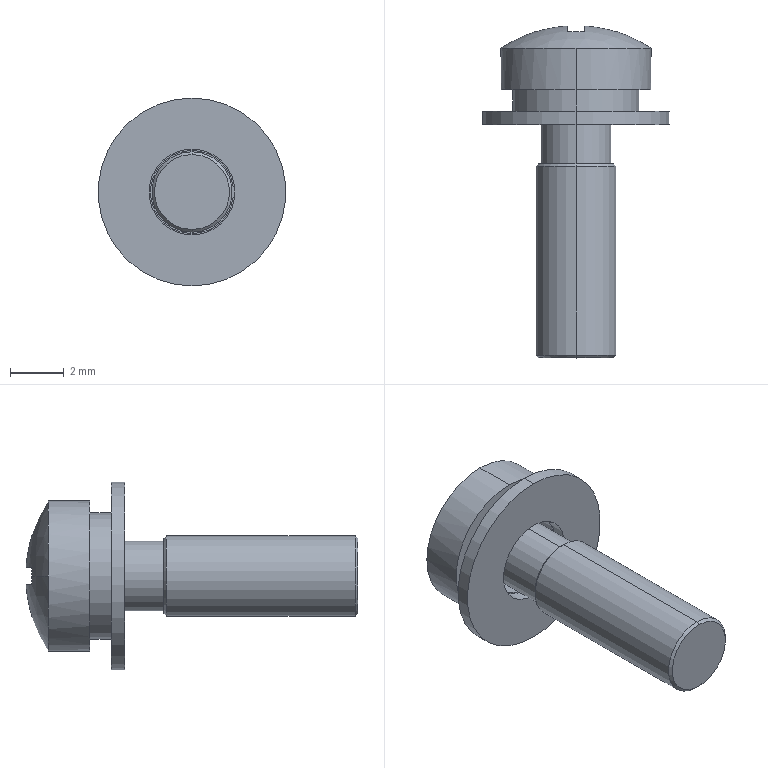Part | STEP file | 3 solids | 46 faces | box 7 x 12.378 x 7 mm | volume 131.512 mm3 | plane 22 | cylinder 16 | cone 4 | torus 2 | sphere 2 | commonest cylinder face diameters 3.1 x3 4.7 x3 2.6 x2 3 x2 3.2 x2 5.6 x2
STEP:
#1=CARTESIAN_POINT('',(0.,-12.4,-1.4));
#2=VERTEX_POINT('',#1);
#3=CARTESIAN_POINT('',(0.,-12.4,1.4));
#4=VERTEX_POINT('',#3);
#5=CARTESIAN_POINT('',(0.,-12.4,0.));
#6=DIRECTION('',(0.,-1.,0.));
#7=DIRECTION('',(0.,0.,1.));
#8=AXIS2_PLACEMENT_3D('',#5,#6,#7);
#9=CIRCLE('',#8,1.4);
#10=EDGE_CURVE('',#2,#4,#9,.T.);
#11=ORIENTED_EDGE('',*,*,#10,.F.);
#12=CARTESIAN_POINT('',(0.,-12.3,-1.5));
#13=VERTEX_POINT('',#12);
#14=CARTESIAN_POINT('',(0.,-12.4,-1.4));
#15=DIRECTION('',(0.,0.7071,-0.7071));
#16=VECTOR('',#15,1000.);
#17=LINE('',#14,#16);
#18=EDGE_CURVE('',#2,#13,#17,.T.);
#19=ORIENTED_EDGE('',*,*,#18,.T.);
#20=CARTESIAN_POINT('',(0.,-12.3,1.5));
#21=VERTEX_POINT('',#20);
#22=CARTESIAN_POINT('',(0.,-12.3,0.));
#23=DIRECTION('',(0.,1.,0.));
#24=DIRECTION('',(0.,0.,1.));
#25=AXIS2_PLACEMENT_3D('',#22,#23,#24);
#26=CIRCLE('',#25,1.5);
#27=EDGE_CURVE('',#21,#13,#26,.T.);
#28=ORIENTED_EDGE('',*,*,#27,.F.);
#29=CARTESIAN_POINT('',(0.,-12.4,1.4));
#30=DIRECTION('',(0.,0.7071,0.7071));
#31=VECTOR('',#30,1000.);
#32=LINE('',#29,#31);
#33=EDGE_CURVE('',#4,#21,#32,.T.);
#34=ORIENTED_EDGE('',*,*,#33,.F.);
#35=EDGE_LOOP('',(#11,#19,#28,#34));
#36=FACE_OUTER_BOUND('',#35,.T.);
#37=CARTESIAN_POINT('',(0.,-12.4,0.));
#38=DIRECTION('',(0.,1.,0.));
#39=DIRECTION('',(0.,0.,1.));
#40=AXIS2_PLACEMENT_3D('',#37,#38,#39);
#41=CONICAL_SURFACE('',#40,1.4,0.7854);
#42=ADVANCED_FACE('',(#36),#41,.T.);
#43=CARTESIAN_POINT('',(0.,-5.16,1.4));
#44=VERTEX_POINT('',#43);
#45=CARTESIAN_POINT('',(0.,-5.16,-1.4));
#46=VERTEX_POINT('',#45);
#47=CARTESIAN_POINT('',(0.,-5.16,0.));
#48=DIRECTION('',(0.,1.,0.));
#49=DIRECTION('',(0.,0.,1.));
#50=AXIS2_PLACEMENT_3D('',#47,#48,#49);
#51=CIRCLE('',#50,1.4);
#52=EDGE_CURVE('',#44,#46,#51,.T.);
#53=ORIENTED_EDGE('',*,*,#52,.F.);
#54=CARTESIAN_POINT('',(0.,-5.26,1.5));
#55=VERTEX_POINT('',#54);
#56=CARTESIAN_POINT('',(0.,-5.26,1.5));
#57=DIRECTION('',(0.,-0.7071,0.7071));
#58=VECTOR('',#57,1000.);
#59=LINE('',#56,#58);
#60=EDGE_CURVE('',#44,#55,#59,.T.);
#61=ORIENTED_EDGE('',*,*,#60,.T.);
#62=CARTESIAN_POINT('',(0.,-5.26,-1.5));
#63=VERTEX_POINT('',#62);
#64=CARTESIAN_POINT('',(0.,-5.26,0.));
#65=DIRECTION('',(0.,-1.,0.));
#66=DIRECTION('',(0.,0.,1.));
#67=AXIS2_PLACEMENT_3D('',#64,#65,#66);
#68=CIRCLE('',#67,1.5);
#69=EDGE_CURVE('',#63,#55,#68,.T.);
#70=ORIENTED_EDGE('',*,*,#69,.F.);
#71=CARTESIAN_POINT('',(0.,-5.26,-1.5));
#72=DIRECTION('',(0.,-0.7071,-0.7071));
#73=VECTOR('',#72,1000.);
#74=LINE('',#71,#73);
#75=EDGE_CURVE('',#46,#63,#74,.T.);
#76=ORIENTED_EDGE('',*,*,#75,.F.);
#77=EDGE_LOOP('',(#53,#61,#70,#76));
#78=FACE_OUTER_BOUND('',#77,.T.);
#79=CARTESIAN_POINT('',(0.,-5.26,0.));
#80=DIRECTION('',(0.,-1.,0.));
#81=DIRECTION('',(0.,0.,-1.));
#82=AXIS2_PLACEMENT_3D('',#79,#80,#81);
#83=CONICAL_SURFACE('',#82,1.5,0.7854);
#84=ADVANCED_FACE('',(#78),#83,.T.);
#85=CARTESIAN_POINT('',(0.,-2.5,1.3));
#86=VERTEX_POINT('',#85);
#87=CARTESIAN_POINT('',(0.,-2.5,-1.3));
#88=VERTEX_POINT('',#87);
#89=CARTESIAN_POINT('',(0.,-2.5,0.));
#90=DIRECTION('',(0.,-1.,0.));
#91=DIRECTION('',(0.,0.,-1.));
#92=AXIS2_PLACEMENT_3D('',#89,#90,#91);
#93=CIRCLE('',#92,1.3);
#94=EDGE_CURVE('',#86,#88,#93,.T.);
#95=ORIENTED_EDGE('',*,*,#94,.F.);
#96=CARTESIAN_POINT('',(0.,-2.4,1.4));
#97=VERTEX_POINT('',#96);
#98=CARTESIAN_POINT('',(0.,-2.5,1.4));
#99=DIRECTION('',(1.,0.,0.));
#100=DIRECTION('',(0.,0.,-1.));
#101=AXIS2_PLACEMENT_3D('',#98,#99,#100);
#102=CIRCLE('',#101,0.1);
#103=EDGE_CURVE('',#86,#97,#102,.T.);
#104=ORIENTED_EDGE('',*,*,#103,.T.);
#105=CARTESIAN_POINT('',(0.,-2.4,-1.4));
#106=VERTEX_POINT('',#105);
#107=CARTESIAN_POINT('',(0.,-2.4,0.));
#108=DIRECTION('',(0.,1.,0.));
#109=DIRECTION('',(0.,0.,-1.));
#110=AXIS2_PLACEMENT_3D('',#107,#108,#109);
#111=CIRCLE('',#110,1.4);
#112=EDGE_CURVE('',#106,#97,#111,.T.);
#113=ORIENTED_EDGE('',*,*,#112,.F.);
#114=CARTESIAN_POINT('',(0.,-2.5,-1.4));
#115=DIRECTION('',(-1.,0.,0.));
#116=DIRECTION('',(0.,0.,1.));
#117=AXIS2_PLACEMENT_3D('',#114,#115,#116);
#118=CIRCLE('',#117,0.1);
#119=EDGE_CURVE('',#88,#106,#118,.T.);
#120=ORIENTED_EDGE('',*,*,#119,.F.);
#121=EDGE_LOOP('',(#95,#104,#113,#120));
#122=FACE_OUTER_BOUND('',#121,.T.);
#123=CARTESIAN_POINT('',(0.,-2.5,0.));
#124=DIRECTION('',(0.,-1.,0.));
#125=DIRECTION('',(0.,0.,-1.));
#126=AXIS2_PLACEMENT_3D('',#123,#124,#125);
#127=TOROIDAL_SURFACE('',#126,1.4,0.1);
#128=ADVANCED_FACE('',(#122),#127,.F.);
#129=CARTESIAN_POINT('',(-1.5,-0.2303,0.));
#130=VERTEX_POINT('',#129);
#131=CARTESIAN_POINT('',(-1.5,-0.2421,0.335));
#132=VERTEX_POINT('',#131);
#133=CARTESIAN_POINT('',(-1.5,-5.,0.));
#134=DIRECTION('',(1.,0.,0.));
#135=DIRECTION('',(0.,0.,1.));
#136=AXIS2_PLACEMENT_3D('',#133,#134,#135);
#137=CIRCLE('',#136,4.77);
#138=EDGE_CURVE('',#130,#132,#137,.T.);
#139=ORIENTED_EDGE('',*,*,#138,.F.);
#140=CARTESIAN_POINT('',(-2.8,-0.8575,0.));
#141=VERTEX_POINT('',#140);
#142=CARTESIAN_POINT('',(0.,-5.,0.));
#143=DIRECTION('',(0.,0.,1.));
#144=DIRECTION('',(1.,0.,0.));
#145=AXIS2_PLACEMENT_3D('',#142,#143,#144);
#146=CIRCLE('',#145,5.);
#147=EDGE_CURVE('',#130,#141,#146,.T.);
#148=ORIENTED_EDGE('',*,*,#147,.T.);
#149=CARTESIAN_POINT('',(0.,-0.8575,2.8));
#150=VERTEX_POINT('',#149);
#151=CARTESIAN_POINT('',(0.,-0.8575,0.));
#152=DIRECTION('',(0.,-1.,0.));
#153=DIRECTION('',(0.,0.,-1.));
#154=AXIS2_PLACEMENT_3D('',#151,#152,#153);
#155=CIRCLE('',#154,2.8);
#156=EDGE_CURVE('',#150,#141,#155,.T.);
#157=ORIENTED_EDGE('',*,*,#156,.F.);
#158=CARTESIAN_POINT('',(2.8,-0.8575,0.));
#159=VERTEX_POINT('',#158);
#160=CARTESIAN_POINT('',(0.,-0.8575,0.));
#161=DIRECTION('',(0.,-1.,0.));
#162=DIRECTION('',(0.,0.,-1.));
#163=AXIS2_PLACEMENT_3D('',#160,#161,#162);
#164=CIRCLE('',#163,2.8);
#165=EDGE_CURVE('',#159,#150,#164,.T.);
#166=ORIENTED_EDGE('',*,*,#165,.F.);
#167=CARTESIAN_POINT('',(1.5,-0.2303,0.));
#168=VERTEX_POINT('',#167);
#169=CARTESIAN_POINT('',(0.,-5.,0.));
#170=DIRECTION('',(0.,0.,-1.));
#171=DIRECTION('',(-1.,0.,0.));
#172=AXIS2_PLACEMENT_3D('',#169,#170,#171);
#173=CIRCLE('',#172,5.);
#174=EDGE_CURVE('',#168,#159,#173,.T.);
#175=ORIENTED_EDGE('',*,*,#174,.F.);
#176=CARTESIAN_POINT('',(1.5,-0.2421,0.335));
#177=VERTEX_POINT('',#176);
#178=CARTESIAN_POINT('',(1.5,-5.,0.));
#179=DIRECTION('',(-1.,0.,0.));
#180=DIRECTION('',(0.,0.,-1.));
#181=AXIS2_PLACEMENT_3D('',#178,#179,#180);
#182=CIRCLE('',#181,4.77);
#183=EDGE_CURVE('',#177,#168,#182,.T.);
#184=ORIENTED_EDGE('',*,*,#183,.F.);
#185=CARTESIAN_POINT('',(0.335,-0.0225,0.335));
#186=VERTEX_POINT('',#185);
#187=CARTESIAN_POINT('',(0.,-5.,0.335));
#188=DIRECTION('',(0.,0.,-1.));
#189=DIRECTION('',(1.,0.,0.));
#190=AXIS2_PLACEMENT_3D('',#187,#188,#189);
#191=CIRCLE('',#190,4.989);
#192=EDGE_CURVE('',#186,#177,#191,.T.);
#193=ORIENTED_EDGE('',*,*,#192,.F.);
#194=CARTESIAN_POINT('',(0.335,-0.2421,1.5));
#195=VERTEX_POINT('',#194);
#196=CARTESIAN_POINT('',(0.335,-5.,0.));
#197=DIRECTION('',(-1.,0.,0.));
#198=DIRECTION('',(0.,0.,-1.));
#199=AXIS2_PLACEMENT_3D('',#196,#197,#198);
#200=CIRCLE('',#199,4.989);
#201=EDGE_CURVE('',#195,#186,#200,.T.);
#202=ORIENTED_EDGE('',*,*,#201,.F.);
#203=CARTESIAN_POINT('',(-0.335,-0.2421,1.5));
#204=VERTEX_POINT('',#203);
#205=CARTESIAN_POINT('',(0.,-5.,1.5));
#206=DIRECTION('',(0.,0.,-1.));
#207=DIRECTION('',(1.,0.,0.));
#208=AXIS2_PLACEMENT_3D('',#205,#206,#207);
#209=CIRCLE('',#208,4.77);
#210=EDGE_CURVE('',#204,#195,#209,.T.);
#211=ORIENTED_EDGE('',*,*,#210,.F.);
#212=CARTESIAN_POINT('',(-0.335,-0.0225,0.335));
#213=VERTEX_POINT('',#212);
#214=CARTESIAN_POINT('',(-0.335,-5.,0.));
#215=DIRECTION('',(1.,0.,0.));
#216=DIRECTION('',(0.,0.,1.));
#217=AXIS2_PLACEMENT_3D('',#214,#215,#216);
#218=CIRCLE('',#217,4.989);
#219=EDGE_CURVE('',#213,#204,#218,.T.);
#220=ORIENTED_EDGE('',*,*,#219,.F.);
#221=CARTESIAN_POINT('',(0.,-5.,0.335));
#222=DIRECTION('',(0.,0.,-1.));
#223=DIRECTION('',(1.,0.,0.));
#224=AXIS2_PLACEMENT_3D('',#221,#222,#223);
#225=CIRCLE('',#224,4.989);
#226=EDGE_CURVE('',#132,#213,#225,.T.);
#227=ORIENTED_EDGE('',*,*,#226,.F.);
#228=EDGE_LOOP('',(#139,#148,#157,#166,#175,#184,#193,#202,#211,#220,#227));
#229=FACE_OUTER_BOUND('',#228,.T.);
#230=CARTESIAN_POINT('',(0.,-5.,0.));
#231=DIRECTION('',(0.,0.,1.));
#232=DIRECTION('',(1.,0.,0.));
#233=AXIS2_PLACEMENT_3D('',#230,#231,#232);
#234=SPHERICAL_SURFACE('',#233,5.);
#235=ADVANCED_FACE('',(#229),#234,.T.);
#236=CARTESIAN_POINT('',(0.,-0.8575,-2.8));
#237=VERTEX_POINT('',#236);
#238=CARTESIAN_POINT('',(0.,-0.8575,0.));
#239=DIRECTION('',(0.,-1.,0.));
#240=DIRECTION('',(0.,0.,-1.));
#241=AXIS2_PLACEMENT_3D('',#238,#239,#240);
#242=CIRCLE('',#241,2.8);
#243=EDGE_CURVE('',#237,#159,#242,.T.);
#244=ORIENTED_EDGE('',*,*,#243,.T.);
#245=ORIENTED_EDGE('',*,*,#165,.T.);
#246=CARTESIAN_POINT('',(0.,-2.4,2.8));
#247=VERTEX_POINT('',#246);
#248=CARTESIAN_POINT('',(0.,-12.4,2.8));
#249=DIRECTION('',(0.,-1.,0.));
#250=VECTOR('',#249,1000.);
#251=LINE('',#248,#250);
#252=EDGE_CURVE('',#150,#247,#251,.T.);
#253=ORIENTED_EDGE('',*,*,#252,.T.);
#254=CARTESIAN_POINT('',(0.,-2.4,-2.8));
#255=VERTEX_POINT('',#254);
#256=CARTESIAN_POINT('',(0.,-2.4,0.));
#257=DIRECTION('',(0.,-1.,0.));
#258=DIRECTION('',(0.,0.,-1.));
#259=AXIS2_PLACEMENT_3D('',#256,#257,#258);
#260=CIRCLE('',#259,2.8);
#261=EDGE_CURVE('',#255,#247,#260,.T.);
#262=ORIENTED_EDGE('',*,*,#261,.F.);
#263=CARTESIAN_POINT('',(0.,-12.4,-2.8));
#264=DIRECTION('',(0.,-1.,0.));
#265=VECTOR('',#264,1000.);
#266=LINE('',#263,#265);
#267=EDGE_CURVE('',#237,#255,#266,.T.);
#268=ORIENTED_EDGE('',*,*,#267,.F.);
#269=EDGE_LOOP('',(#244,#245,#253,#262,#268));
#270=FACE_OUTER_BOUND('',#269,.T.);
#271=CARTESIAN_POINT('',(0.,-12.4,0.));
#272=DIRECTION('',(0.,-1.,0.));
#273=DIRECTION('',(0.,0.,-1.));
#274=AXIS2_PLACEMENT_3D('',#271,#272,#273);
#275=CYLINDRICAL_SURFACE('',#274,2.8);
#276=ADVANCED_FACE('',(#270),#275,.T.);
#277=CARTESIAN_POINT('',(0.,-2.5,0.));
#278=DIRECTION('',(0.,-1.,0.));
#279=DIRECTION('',(0.,0.,-1.));
#280=AXIS2_PLACEMENT_3D('',#277,#278,#279);
#281=CIRCLE('',#280,1.3);
#282=EDGE_CURVE('',#88,#86,#281,.T.);
#283=ORIENTED_EDGE('',*,*,#282,.T.);
#284=CARTESIAN_POINT('',(0.,-5.16,1.3));
#285=VERTEX_POINT('',#284);
#286=CARTESIAN_POINT('',(0.,-12.4,1.3));
#287=DIRECTION('',(0.,-1.,0.));
#288=VECTOR('',#287,1000.);
#289=LINE('',#286,#288);
#290=EDGE_CURVE('',#86,#285,#289,.T.);
#291=ORIENTED_EDGE('',*,*,#290,.T.);
#292=CARTESIAN_POINT('',(0.,-5.16,-1.3));
#293=VERTEX_POINT('',#292);
#294=CARTESIAN_POINT('',(0.,-5.16,0.));
#295=DIRECTION('',(0.,-1.,0.));
#296=DIRECTION('',(0.,0.,-1.));
#297=AXIS2_PLACEMENT_3D('',#294,#295,#296);
#298=CIRCLE('',#297,1.3);
#299=EDGE_CURVE('',#293,#285,#298,.T.);
#300=ORIENTED_EDGE('',*,*,#299,.F.);
#301=CARTESIAN_POINT('',(0.,-12.4,-1.3));
#302=DIRECTION('',(0.,-1.,0.));
#303=VECTOR('',#302,1000.);
#304=LINE('',#301,#303);
#305=EDGE_CURVE('',#88,#293,#304,.T.);
#306=ORIENTED_EDGE('',*,*,#305,.F.);
#307=EDGE_LOOP('',(#283,#291,#300,#306));
#308=FACE_OUTER_BOUND('',#307,.T.);
#309=CARTESIAN_POINT('',(0.,-12.4,0.));
#310=DIRECTION('',(0.,-1.,0.));
#311=DIRECTION('',(0.,0.,-1.));
#312=AXIS2_PLACEMENT_3D('',#309,#310,#311);
#313=CYLINDRICAL_SURFACE('',#312,1.3);
#314=ADVANCED_FACE('',(#308),#313,.T.);
#315=ORIENTED_EDGE('',*,*,#69,.T.);
#316=CARTESIAN_POINT('',(0.,-12.4,1.5));
#317=DIRECTION('',(0.,-1.,0.));
#318=VECTOR('',#317,1000.);
#319=LINE('',#316,#318);
#320=EDGE_CURVE('',#55,#21,#319,.T.);
#321=ORIENTED_EDGE('',*,*,#320,.T.);
#322=ORIENTED_EDGE('',*,*,#27,.T.);
#323=CARTESIAN_POINT('',(0.,-12.4,-1.5));
#324=DIRECTION('',(0.,-1.,0.));
#325=VECTOR('',#324,1000.);
#326=LINE('',#323,#325);
#327=EDGE_CURVE('',#63,#13,#326,.T.);
#328=ORIENTED_EDGE('',*,*,#327,.F.);
#329=EDGE_LOOP('',(#315,#321,#322,#328));
#330=FACE_OUTER_BOUND('',#329,.T.);
#331=CARTESIAN_POINT('',(0.,-12.4,0.));
#332=DIRECTION('',(0.,-1.,0.));
#333=DIRECTION('',(0.,0.,-1.));
#334=AXIS2_PLACEMENT_3D('',#331,#332,#333);
#335=CYLINDRICAL_SURFACE('',#334,1.5);
#336=ADVANCED_FACE('',(#330),#335,.T.);
#337=CARTESIAN_POINT('',(0.,-12.4,0.));
#338=DIRECTION('',(0.,-1.,0.));
#339=DIRECTION('',(0.,0.,1.));
#340=AXIS2_PLACEMENT_3D('',#337,#338,#339);
#341=CIRCLE('',#340,1.4);
#342=EDGE_CURVE('',#4,#2,#341,.T.);
#343=ORIENTED_EDGE('',*,*,#342,.T.);
#344=ORIENTED_EDGE('',*,*,#10,.T.);
#345=EDGE_LOOP('',(#343,#344));
#346=FACE_OUTER_BOUND('',#345,.T.);
#347=CARTESIAN_POINT('',(0.,-12.4,0.));
#348=DIRECTION('',(0.,1.,0.));
#349=DIRECTION('',(0.,0.,1.));
#350=AXIS2_PLACEMENT_3D('',#347,#348,#349);
#351=PLANE('',#350);
#352=ADVANCED_FACE('',(#346),#351,.F.);
#353=ORIENTED_EDGE('',*,*,#320,.F.);
#354=CARTESIAN_POINT('',(0.,-5.26,0.));
#355=DIRECTION('',(0.,-1.,0.));
#356=DIRECTION('',(0.,0.,1.));
#357=AXIS2_PLACEMENT_3D('',#354,#355,#356);
#358=CIRCLE('',#357,1.5);
#359=EDGE_CURVE('',#55,#63,#358,.T.);
#360=ORIENTED_EDGE('',*,*,#359,.T.);
#361=ORIENTED_EDGE('',*,*,#327,.T.);
#362=CARTESIAN_POINT('',(0.,-12.3,0.));
#363=DIRECTION('',(0.,1.,0.));
#364=DIRECTION('',(0.,0.,1.));
#365=AXIS2_PLACEMENT_3D('',#362,#363,#364);
#366=CIRCLE('',#365,1.5);
#367=EDGE_CURVE('',#13,#21,#366,.T.);
#368=ORIENTED_EDGE('',*,*,#367,.T.);
#369=EDGE_LOOP('',(#353,#360,#361,#368));
#370=FACE_OUTER_BOUND('',#369,.T.);
#371=CARTESIAN_POINT('',(0.,-12.4,0.));
#372=DIRECTION('',(0.,-1.,0.));
#373=DIRECTION('',(0.,0.,-1.));
#374=AXIS2_PLACEMENT_3D('',#371,#372,#373);
#375=CYLINDRICAL_SURFACE('',#374,1.5);
#376=ADVANCED_FACE('',(#370),#375,.T.);
#377=CARTESIAN_POINT('',(0.,-5.16,0.));
#378=DIRECTION('',(0.,1.,0.));
#379=DIRECTION('',(0.,0.,1.));
#380=AXIS2_PLACEMENT_3D('',#377,#378,#379);
#381=CIRCLE('',#380,1.4);
#382=EDGE_CURVE('',#46,#44,#381,.T.);
#383=ORIENTED_EDGE('',*,*,#382,.T.);
#384=ORIENTED_EDGE('',*,*,#52,.T.);
#385=EDGE_LOOP('',(#383,#384));
#386=FACE_OUTER_BOUND('',#385,.T.);
#387=ORIENTED_EDGE('',*,*,#299,.T.);
#388=CARTESIAN_POINT('',(0.,-5.16,0.));
#389=DIRECTION('',(0.,-1.,0.));
#390=DIRECTION('',(0.,0.,-1.));
#391=AXIS2_PLACEMENT_3D('',#388,#389,#390);
#392=CIRCLE('',#391,1.3);
#393=EDGE_CURVE('',#285,#293,#392,.T.);
#394=ORIENTED_EDGE('',*,*,#393,.T.);
#395=EDGE_LOOP('',(#387,#394));
#396=FACE_BOUND('',#395,.T.);
#397=CARTESIAN_POINT('',(0.,-5.16,0.));
#398=DIRECTION('',(0.,1.,0.));
#399=DIRECTION('',(0.,0.,1.));
#400=AXIS2_PLACEMENT_3D('',#397,#398,#399);
#401=PLANE('',#400);
#402=ADVANCED_FACE('',(#386,#396),#401,.T.);
#403=ORIENTED_EDGE('',*,*,#290,.F.);
#404=ORIENTED_EDGE('',*,*,#94,.T.);
#405=ORIENTED_EDGE('',*,*,#305,.T.);
#406=ORIENTED_EDGE('',*,*,#393,.F.);
#407=EDGE_LOOP('',(#403,#404,#405,#406));
#408=FACE_OUTER_BOUND('',#407,.T.);
#409=CARTESIAN_POINT('',(0.,-12.4,0.));
#410=DIRECTION('',(0.,-1.,0.));
#411=DIRECTION('',(0.,0.,-1.));
#412=AXIS2_PLACEMENT_3D('',#409,#410,#411);
#413=CYLINDRICAL_SURFACE('',#412,1.3);
#414=ADVANCED_FACE('',(#408),#413,.T.);
#415=ORIENTED_EDGE('',*,*,#112,.T.);
#416=CARTESIAN_POINT('',(0.,-2.4,0.));
#417=DIRECTION('',(0.,1.,0.));
#418=DIRECTION('',(0.,0.,-1.));
#419=AXIS2_PLACEMENT_3D('',#416,#417,#418);
#420=CIRCLE('',#419,1.4);
#421=EDGE_CURVE('',#97,#106,#420,.T.);
#422=ORIENTED_EDGE('',*,*,#421,.T.);
#423=EDGE_LOOP('',(#415,#422));
#424=FACE_BOUND('',#423,.T.);
#425=ORIENTED_EDGE('',*,*,#261,.T.);
#426=CARTESIAN_POINT('',(0.,-2.4,0.));
#427=DIRECTION('',(0.,-1.,0.));
#428=DIRECTION('',(0.,0.,-1.));
#429=AXIS2_PLACEMENT_3D('',#426,#427,#428);
#430=CIRCLE('',#429,2.8);
#431=EDGE_CURVE('',#247,#255,#430,.T.);
#432=ORIENTED_EDGE('',*,*,#431,.T.);
#433=EDGE_LOOP('',(#425,#432));
#434=FACE_OUTER_BOUND('',#433,.T.);
#435=CARTESIAN_POINT('',(0.,-2.4,0.));
#436=DIRECTION('',(0.,-1.,0.));
#437=DIRECTION('',(0.,0.,-1.));
#438=AXIS2_PLACEMENT_3D('',#435,#436,#437);
#439=PLANE('',#438);
#440=ADVANCED_FACE('',(#424,#434),#439,.T.);
#441=ORIENTED_EDGE('',*,*,#252,.F.);
#442=ORIENTED_EDGE('',*,*,#156,.T.);
#443=CARTESIAN_POINT('',(0.,-0.8575,0.));
#444=DIRECTION('',(0.,-1.,0.));
#445=DIRECTION('',(0.,0.,-1.));
#446=AXIS2_PLACEMENT_3D('',#443,#444,#445);
#447=CIRCLE('',#446,2.8);
#448=EDGE_CURVE('',#141,#237,#447,.T.);
#449=ORIENTED_EDGE('',*,*,#448,.T.);
#450=ORIENTED_EDGE('',*,*,#267,.T.);
#451=ORIENTED_EDGE('',*,*,#431,.F.);
#452=EDGE_LOOP('',(#441,#442,#449,#450,#451));
#453=FACE_OUTER_BOUND('',#452,.T.);
#454=CARTESIAN_POINT('',(0.,-12.4,0.));
#455=DIRECTION('',(0.,-1.,0.));
#456=DIRECTION('',(0.,0.,-1.));
#457=AXIS2_PLACEMENT_3D('',#454,#455,#456);
#458=CYLINDRICAL_SURFACE('',#457,2.8);
#459=ADVANCED_FACE('',(#453),#458,.T.);
#460=ORIENTED_EDGE('',*,*,#147,.F.);
#461=CARTESIAN_POINT('',(-1.5,-0.2421,-0.335));
#462=VERTEX_POINT('',#461);
#463=CARTESIAN_POINT('',(-1.5,-5.,0.));
#464=DIRECTION('',(1.,0.,0.));
#465=DIRECTION('',(0.,0.,1.));
#466=AXIS2_PLACEMENT_3D('',#463,#464,#465);
#467=CIRCLE('',#466,4.77);
#468=EDGE_CURVE('',#462,#130,#467,.T.);
#469=ORIENTED_EDGE('',*,*,#468,.F.);
#470=CARTESIAN_POINT('',(-0.335,-0.0225,-0.335));
#471=VERTEX_POINT('',#470);
#472=CARTESIAN_POINT('',(0.,-5.,-0.335));
#473=DIRECTION('',(0.,0.,1.));
#474=DIRECTION('',(-1.,0.,0.));
#475=AXIS2_PLACEMENT_3D('',#472,#473,#474);
#476=CIRCLE('',#475,4.989);
#477=EDGE_CURVE('',#471,#462,#476,.T.);
#478=ORIENTED_EDGE('',*,*,#477,.F.);
#479=CARTESIAN_POINT('',(-0.335,-0.2421,-1.5));
#480=VERTEX_POINT('',#479);
#481=CARTESIAN_POINT('',(-0.335,-5.,0.));
#482=DIRECTION('',(1.,0.,0.));
#483=DIRECTION('',(0.,0.,1.));
#484=AXIS2_PLACEMENT_3D('',#481,#482,#483);
#485=CIRCLE('',#484,4.989);
#486=EDGE_CURVE('',#480,#471,#485,.T.);
#487=ORIENTED_EDGE('',*,*,#486,.F.);
#488=CARTESIAN_POINT('',(0.335,-0.2421,-1.5));
#489=VERTEX_POINT('',#488);
#490=CARTESIAN_POINT('',(0.,-5.,-1.5));
#491=DIRECTION('',(0.,0.,1.));
#492=DIRECTION('',(-1.,0.,0.));
#493=AXIS2_PLACEMENT_3D('',#490,#491,#492);
#494=CIRCLE('',#493,4.77);
#495=EDGE_CURVE('',#489,#480,#494,.T.);
#496=ORIENTED_EDGE('',*,*,#495,.F.);
#497=CARTESIAN_POINT('',(0.335,-0.0225,-0.335));
#498=VERTEX_POINT('',#497);
#499=CARTESIAN_POINT('',(0.335,-5.,0.));
#500=DIRECTION('',(-1.,0.,0.));
#501=DIRECTION('',(0.,0.,-1.));
#502=AXIS2_PLACEMENT_3D('',#499,#500,#501);
#503=CIRCLE('',#502,4.989);
#504=EDGE_CURVE('',#498,#489,#503,.T.);
#505=ORIENTED_EDGE('',*,*,#504,.F.);
#506=CARTESIAN_POINT('',(1.5,-0.2421,-0.335));
#507=VERTEX_POINT('',#506);
#508=CARTESIAN_POINT('',(0.,-5.,-0.335));
#509=DIRECTION('',(0.,0.,1.));
#510=DIRECTION('',(-1.,0.,0.));
#511=AXIS2_PLACEMENT_3D('',#508,#509,#510);
#512=CIRCLE('',#511,4.989);
#513=EDGE_CURVE('',#507,#498,#512,.T.);
#514=ORIENTED_EDGE('',*,*,#513,.F.);
#515=CARTESIAN_POINT('',(1.5,-5.,0.));
#516=DIRECTION('',(-1.,0.,0.));
#517=DIRECTION('',(0.,0.,-1.));
#518=AXIS2_PLACEMENT_3D('',#515,#516,#517);
#519=CIRCLE('',#518,4.77);
#520=EDGE_CURVE('',#168,#507,#519,.T.);
#521=ORIENTED_EDGE('',*,*,#520,.F.);
#522=ORIENTED_EDGE('',*,*,#174,.T.);
#523=ORIENTED_EDGE('',*,*,#243,.F.);
#524=ORIENTED_EDGE('',*,*,#448,.F.);
#525=EDGE_LOOP('',(#460,#469,#478,#487,#496,#505,#514,#521,#522,#523,#524));
#526=FACE_OUTER_BOUND('',#525,.T.);
#527=CARTESIAN_POINT('',(0.,-5.,0.));
#528=DIRECTION('',(0.,0.,1.));
#529=DIRECTION('',(1.,0.,0.));
#530=AXIS2_PLACEMENT_3D('',#527,#528,#529);
#531=SPHERICAL_SURFACE('',#530,5.);
#532=ADVANCED_FACE('',(#526),#531,.T.);
#533=ORIENTED_EDGE('',*,*,#513,.T.);
#534=CARTESIAN_POINT('',(0.335,-1.75,-0.335));
#535=VERTEX_POINT('',#534);
#536=CARTESIAN_POINT('',(0.335,-1.75,-0.335));
#537=DIRECTION('',(0.,1.,0.));
#538=VECTOR('',#537,1000.);
#539=LINE('',#536,#538);
#540=EDGE_CURVE('',#535,#498,#539,.T.);
#541=ORIENTED_EDGE('',*,*,#540,.F.);
#542=CARTESIAN_POINT('',(1.5,-1.75,-0.335));
#543=VERTEX_POINT('',#542);
#544=CARTESIAN_POINT('',(0.335,-1.75,-0.335));
#545=DIRECTION('',(-1.,0.,0.));
#546=VECTOR('',#545,1000.);
#547=LINE('',#544,#546);
#548=EDGE_CURVE('',#543,#535,#547,.T.);
#549=ORIENTED_EDGE('',*,*,#548,.F.);
#550=CARTESIAN_POINT('',(1.5,-1.75,-0.335));
#551=DIRECTION('',(0.,1.,0.));
#552=VECTOR('',#551,1000.);
#553=LINE('',#550,#552);
#554=EDGE_CURVE('',#543,#507,#553,.T.);
#555=ORIENTED_EDGE('',*,*,#554,.T.);
#556=EDGE_LOOP('',(#533,#541,#549,#555));
#557=FACE_OUTER_BOUND('',#556,.T.);
#558=CARTESIAN_POINT('',(0.335,-1.75,-0.335));
#559=DIRECTION('',(0.,0.,-1.));
#560=DIRECTION('',(-1.,0.,0.));
#561=AXIS2_PLACEMENT_3D('',#558,#559,#560);
#562=PLANE('',#561);
#563=ADVANCED_FACE('',(#557),#562,.F.);
#564=ORIENTED_EDGE('',*,*,#183,.T.);
#565=ORIENTED_EDGE('',*,*,#520,.T.);
#566=ORIENTED_EDGE('',*,*,#554,.F.);
#567=CARTESIAN_POINT('',(1.5,-1.75,0.335));
#568=VERTEX_POINT('',#567);
#569=CARTESIAN_POINT('',(1.5,-1.75,-0.335));
#570=DIRECTION('',(0.,0.,-1.));
#571=VECTOR('',#570,1000.);
#572=LINE('',#569,#571);
#573=EDGE_CURVE('',#568,#543,#572,.T.);
#574=ORIENTED_EDGE('',*,*,#573,.F.);
#575=CARTESIAN_POINT('',(1.5,-1.75,0.335));
#576=DIRECTION('',(0.,1.,0.));
#577=VECTOR('',#576,1000.);
#578=LINE('',#575,#577);
#579=EDGE_CURVE('',#568,#177,#578,.T.);
#580=ORIENTED_EDGE('',*,*,#579,.T.);
#581=EDGE_LOOP('',(#564,#565,#566,#574,#580));
#582=FACE_OUTER_BOUND('',#581,.T.);
#583=CARTESIAN_POINT('',(1.5,-1.75,-0.335));
#584=DIRECTION('',(1.,0.,0.));
#585=DIRECTION('',(0.,0.,-1.));
#586=AXIS2_PLACEMENT_3D('',#583,#584,#585);
#587=PLANE('',#586);
#588=ADVANCED_FACE('',(#582),#587,.F.);
#589=ORIENTED_EDGE('',*,*,#192,.T.);
#590=ORIENTED_EDGE('',*,*,#579,.F.);
#591=CARTESIAN_POINT('',(0.335,-1.75,0.335));
#592=VERTEX_POINT('',#591);
#593=CARTESIAN_POINT('',(0.335,-1.75,0.335));
#594=DIRECTION('',(1.,0.,0.));
#595=VECTOR('',#594,1000.);
#596=LINE('',#593,#595);
#597=EDGE_CURVE('',#592,#568,#596,.T.);
#598=ORIENTED_EDGE('',*,*,#597,.F.);
#599=CARTESIAN_POINT('',(0.335,-1.75,0.335));
#600=DIRECTION('',(0.,1.,0.));
#601=VECTOR('',#600,1000.);
#602=LINE('',#599,#601);
#603=EDGE_CURVE('',#592,#186,#602,.T.);
#604=ORIENTED_EDGE('',*,*,#603,.T.);
#605=EDGE_LOOP('',(#589,#590,#598,#604));
#606=FACE_OUTER_BOUND('',#605,.T.);
#607=CARTESIAN_POINT('',(0.335,-1.75,0.335));
#608=DIRECTION('',(0.,0.,1.));
#609=DIRECTION('',(1.,0.,0.));
#610=AXIS2_PLACEMENT_3D('',#607,#608,#609);
#611=PLANE('',#610);
#612=ADVANCED_FACE('',(#606),#611,.F.);
#613=ORIENTED_EDGE('',*,*,#201,.T.);
#614=ORIENTED_EDGE('',*,*,#603,.F.);
#615=CARTESIAN_POINT('',(0.335,-1.75,1.5));
#616=VERTEX_POINT('',#615);
#617=CARTESIAN_POINT('',(0.335,-1.75,1.5));
#618=DIRECTION('',(0.,0.,-1.));
#619=VECTOR('',#618,1000.);
#620=LINE('',#617,#619);
#621=EDGE_CURVE('',#616,#592,#620,.T.);
#622=ORIENTED_EDGE('',*,*,#621,.F.);
#623=CARTESIAN_POINT('',(0.335,-1.75,1.5));
#624=DIRECTION('',(0.,1.,0.));
#625=VECTOR('',#624,1000.);
#626=LINE('',#623,#625);
#627=EDGE_CURVE('',#616,#195,#626,.T.);
#628=ORIENTED_EDGE('',*,*,#627,.T.);
#629=EDGE_LOOP('',(#613,#614,#622,#628));
#630=FACE_OUTER_BOUND('',#629,.T.);
#631=CARTESIAN_POINT('',(0.335,-1.75,1.5));
#632=DIRECTION('',(1.,0.,0.));
#633=DIRECTION('',(0.,0.,-1.));
#634=AXIS2_PLACEMENT_3D('',#631,#632,#633);
#635=PLANE('',#634);
#636=ADVANCED_FACE('',(#630),#635,.F.);
#637=ORIENTED_EDGE('',*,*,#210,.T.);
#638=ORIENTED_EDGE('',*,*,#627,.F.);
#639=CARTESIAN_POINT('',(-0.335,-1.75,1.5));
#640=VERTEX_POINT('',#639);
#641=CARTESIAN_POINT('',(-0.335,-1.75,1.5));
#642=DIRECTION('',(1.,0.,0.));
#643=VECTOR('',#642,1000.);
#644=LINE('',#641,#643);
#645=EDGE_CURVE('',#640,#616,#644,.T.);
#646=ORIENTED_EDGE('',*,*,#645,.F.);
#647=CARTESIAN_POINT('',(-0.335,-1.75,1.5));
#648=DIRECTION('',(0.,1.,0.));
#649=VECTOR('',#648,1000.);
#650=LINE('',#647,#649);
#651=EDGE_CURVE('',#640,#204,#650,.T.);
#652=ORIENTED_EDGE('',*,*,#651,.T.);
#653=EDGE_LOOP('',(#637,#638,#646,#652));
#654=FACE_OUTER_BOUND('',#653,.T.);
#655=CARTESIAN_POINT('',(-0.335,-1.75,1.5));
#656=DIRECTION('',(0.,0.,1.));
#657=DIRECTION('',(1.,0.,0.));
#658=AXIS2_PLACEMENT_3D('',#655,#656,#657);
#659=PLANE('',#658);
#660=ADVANCED_FACE('',(#654),#659,.F.);
#661=ORIENTED_EDGE('',*,*,#219,.T.);
#662=ORIENTED_EDGE('',*,*,#651,.F.);
#663=CARTESIAN_POINT('',(-0.335,-1.75,0.335));
#664=VERTEX_POINT('',#663);
#665=CARTESIAN_POINT('',(-0.335,-1.75,1.5));
#666=DIRECTION('',(0.,0.,1.));
#667=VECTOR('',#666,1000.);
#668=LINE('',#665,#667);
#669=EDGE_CURVE('',#664,#640,#668,.T.);
#670=ORIENTED_EDGE('',*,*,#669,.F.);
#671=CARTESIAN_POINT('',(-0.335,-1.75,0.335));
#672=DIRECTION('',(0.,1.,0.));
#673=VECTOR('',#672,1000.);
#674=LINE('',#671,#673);
#675=EDGE_CURVE('',#664,#213,#674,.T.);
#676=ORIENTED_EDGE('',*,*,#675,.T.);
#677=EDGE_LOOP('',(#661,#662,#670,#676));
#678=FACE_OUTER_BOUND('',#677,.T.);
#679=CARTESIAN_POINT('',(-0.335,-1.75,1.5));
#680=DIRECTION('',(-1.,0.,0.));
#681=DIRECTION('',(0.,0.,1.));
#682=AXIS2_PLACEMENT_3D('',#679,#680,#681);
#683=PLANE('',#682);
#684=ADVANCED_FACE('',(#678),#683,.F.);
#685=ORIENTED_EDGE('',*,*,#226,.T.);
#686=ORIENTED_EDGE('',*,*,#675,.F.);
#687=CARTESIAN_POINT('',(-1.5,-1.75,0.335));
#688=VERTEX_POINT('',#687);
#689=CARTESIAN_POINT('',(-0.335,-1.75,0.335));
#690=DIRECTION('',(1.,0.,0.));
#691=VECTOR('',#690,1000.);
#692=LINE('',#689,#691);
#693=EDGE_CURVE('',#688,#664,#692,.T.);
#694=ORIENTED_EDGE('',*,*,#693,.F.);
#695=CARTESIAN_POINT('',(-1.5,-1.75,0.335));
#696=DIRECTION('',(0.,1.,0.));
#697=VECTOR('',#696,1000.);
#698=LINE('',#695,#697);
#699=EDGE_CURVE('',#688,#132,#698,.T.);
#700=ORIENTED_EDGE('',*,*,#699,.T.);
#701=EDGE_LOOP('',(#685,#686,#694,#700));
#702=FACE_OUTER_BOUND('',#701,.T.);
#703=CARTESIAN_POINT('',(-0.335,-1.75,0.335));
#704=DIRECTION('',(0.,0.,1.));
#705=DIRECTION('',(1.,0.,0.));
#706=AXIS2_PLACEMENT_3D('',#703,#704,#705);
#707=PLANE('',#706);
#708=ADVANCED_FACE('',(#702),#707,.F.);
#709=ORIENTED_EDGE('',*,*,#468,.T.);
#710=ORIENTED_EDGE('',*,*,#138,.T.);
#711=ORIENTED_EDGE('',*,*,#699,.F.);
#712=CARTESIAN_POINT('',(-1.5,-1.75,-0.335));
#713=VERTEX_POINT('',#712);
#714=CARTESIAN_POINT('',(-1.5,-1.75,-0.335));
#715=DIRECTION('',(0.,0.,1.));
#716=VECTOR('',#715,1000.);
#717=LINE('',#714,#716);
#718=EDGE_CURVE('',#713,#688,#717,.T.);
#719=ORIENTED_EDGE('',*,*,#718,.F.);
#720=CARTESIAN_POINT('',(-1.5,-1.75,-0.335));
#721=DIRECTION('',(0.,1.,0.));
#722=VECTOR('',#721,1000.);
#723=LINE('',#720,#722);
#724=EDGE_CURVE('',#713,#462,#723,.T.);
#725=ORIENTED_EDGE('',*,*,#724,.T.);
#726=EDGE_LOOP('',(#709,#710,#711,#719,#725));
#727=FACE_OUTER_BOUND('',#726,.T.);
#728=CARTESIAN_POINT('',(-1.5,-1.75,-0.335));
#729=DIRECTION('',(-1.,0.,0.));
#730=DIRECTION('',(0.,0.,1.));
#731=AXIS2_PLACEMENT_3D('',#728,#729,#730);
#732=PLANE('',#731);
#733=ADVANCED_FACE('',(#727),#732,.F.);
#734=ORIENTED_EDGE('',*,*,#477,.T.);
#735=ORIENTED_EDGE('',*,*,#724,.F.);
#736=CARTESIAN_POINT('',(-0.335,-1.75,-0.335));
#737=VERTEX_POINT('',#736);
#738=CARTESIAN_POINT('',(-0.335,-1.75,-0.335));
#739=DIRECTION('',(-1.,0.,0.));
#740=VECTOR('',#739,1000.);
#741=LINE('',#738,#740);
#742=EDGE_CURVE('',#737,#713,#741,.T.);
#743=ORIENTED_EDGE('',*,*,#742,.F.);
#744=CARTESIAN_POINT('',(-0.335,-1.75,-0.335));
#745=DIRECTION('',(0.,1.,0.));
#746=VECTOR('',#745,1000.);
#747=LINE('',#744,#746);
#748=EDGE_CURVE('',#737,#471,#747,.T.);
#749=ORIENTED_EDGE('',*,*,#748,.T.);
#750=EDGE_LOOP('',(#734,#735,#743,#749));
#751=FACE_OUTER_BOUND('',#750,.T.);
#752=CARTESIAN_POINT('',(-0.335,-1.75,-0.335));
#753=DIRECTION('',(0.,0.,-1.));
#754=DIRECTION('',(-1.,0.,0.));
#755=AXIS2_PLACEMENT_3D('',#752,#753,#754);
#756=PLANE('',#755);
#757=ADVANCED_FACE('',(#751),#756,.F.);
#758=ORIENTED_EDGE('',*,*,#486,.T.);
#759=ORIENTED_EDGE('',*,*,#748,.F.);
#760=CARTESIAN_POINT('',(-0.335,-1.75,-1.5));
#761=VERTEX_POINT('',#760);
#762=CARTESIAN_POINT('',(-0.335,-1.75,-1.5));
#763=DIRECTION('',(0.,0.,1.));
#764=VECTOR('',#763,1000.);
#765=LINE('',#762,#764);
#766=EDGE_CURVE('',#761,#737,#765,.T.);
#767=ORIENTED_EDGE('',*,*,#766,.F.);
#768=CARTESIAN_POINT('',(-0.335,-1.75,-1.5));
#769=DIRECTION('',(0.,1.,0.));
#770=VECTOR('',#769,1000.);
#771=LINE('',#768,#770);
#772=EDGE_CURVE('',#761,#480,#771,.T.);
#773=ORIENTED_EDGE('',*,*,#772,.T.);
#774=EDGE_LOOP('',(#758,#759,#767,#773));
#775=FACE_OUTER_BOUND('',#774,.T.);
#776=CARTESIAN_POINT('',(-0.335,-1.75,-1.5));
#777=DIRECTION('',(-1.,0.,0.));
#778=DIRECTION('',(0.,0.,1.));
#779=AXIS2_PLACEMENT_3D('',#776,#777,#778);
#780=PLANE('',#779);
#781=ADVANCED_FACE('',(#775),#780,.F.);
#782=ORIENTED_EDGE('',*,*,#495,.T.);
#783=ORIENTED_EDGE('',*,*,#772,.F.);
#784=CARTESIAN_POINT('',(0.335,-1.75,-1.5));
#785=VERTEX_POINT('',#784);
#786=CARTESIAN_POINT('',(-0.335,-1.75,-1.5));
#787=DIRECTION('',(-1.,0.,0.));
#788=VECTOR('',#787,1000.);
#789=LINE('',#786,#788);
#790=EDGE_CURVE('',#785,#761,#789,.T.);
#791=ORIENTED_EDGE('',*,*,#790,.F.);
#792=CARTESIAN_POINT('',(0.335,-1.75,-1.5));
#793=DIRECTION('',(0.,1.,0.));
#794=VECTOR('',#793,1000.);
#795=LINE('',#792,#794);
#796=EDGE_CURVE('',#785,#489,#795,.T.);
#797=ORIENTED_EDGE('',*,*,#796,.T.);
#798=EDGE_LOOP('',(#782,#783,#791,#797));
#799=FACE_OUTER_BOUND('',#798,.T.);
#800=CARTESIAN_POINT('',(-0.335,-1.75,-1.5));
#801=DIRECTION('',(0.,0.,-1.));
#802=DIRECTION('',(-1.,0.,0.));
#803=AXIS2_PLACEMENT_3D('',#800,#801,#802);
#804=PLANE('',#803);
#805=ADVANCED_FACE('',(#799),#804,.F.);
#806=ORIENTED_EDGE('',*,*,#504,.T.);
#807=ORIENTED_EDGE('',*,*,#796,.F.);
#808=CARTESIAN_POINT('',(0.335,-1.75,-1.5));
#809=DIRECTION('',(0.,0.,-1.));
#810=VECTOR('',#809,1000.);
#811=LINE('',#808,#810);
#812=EDGE_CURVE('',#535,#785,#811,.T.);
#813=ORIENTED_EDGE('',*,*,#812,.F.);
#814=ORIENTED_EDGE('',*,*,#540,.T.);
#815=EDGE_LOOP('',(#806,#807,#813,#814));
#816=FACE_OUTER_BOUND('',#815,.T.);
#817=CARTESIAN_POINT('',(0.335,-1.75,-1.5));
#818=DIRECTION('',(1.,0.,0.));
#819=DIRECTION('',(0.,0.,-1.));
#820=AXIS2_PLACEMENT_3D('',#817,#818,#819);
#821=PLANE('',#820);
#822=ADVANCED_FACE('',(#816),#821,.F.);
#823=ORIENTED_EDGE('',*,*,#548,.T.);
#824=ORIENTED_EDGE('',*,*,#812,.T.);
#825=ORIENTED_EDGE('',*,*,#790,.T.);
#826=ORIENTED_EDGE('',*,*,#766,.T.);
#827=ORIENTED_EDGE('',*,*,#742,.T.);
#828=ORIENTED_EDGE('',*,*,#718,.T.);
#829=ORIENTED_EDGE('',*,*,#693,.T.);
#830=ORIENTED_EDGE('',*,*,#669,.T.);
#831=ORIENTED_EDGE('',*,*,#645,.T.);
#832=ORIENTED_EDGE('',*,*,#621,.T.);
#833=ORIENTED_EDGE('',*,*,#597,.T.);
#834=ORIENTED_EDGE('',*,*,#573,.T.);
#835=EDGE_LOOP('',(#823,#824,#825,#826,#827,#828,#829,#830,#831,#832,#833,#834));
#836=FACE_OUTER_BOUND('',#835,.T.);
#837=CARTESIAN_POINT('',(0.,-1.75,0.));
#838=DIRECTION('',(0.,-1.,0.));
#839=DIRECTION('',(0.,0.,-1.));
#840=AXIS2_PLACEMENT_3D('',#837,#838,#839);
#841=PLANE('',#840);
#842=ADVANCED_FACE('',(#836),#841,.F.);
#843=ORIENTED_EDGE('',*,*,#103,.F.);
#844=ORIENTED_EDGE('',*,*,#282,.F.);
#845=ORIENTED_EDGE('',*,*,#119,.T.);
#846=ORIENTED_EDGE('',*,*,#421,.F.);
#847=EDGE_LOOP('',(#843,#844,#845,#846));
#848=FACE_OUTER_BOUND('',#847,.T.);
#849=CARTESIAN_POINT('',(0.,-2.5,0.));
#850=DIRECTION('',(0.,-1.,0.));
#851=DIRECTION('',(0.,0.,-1.));
#852=AXIS2_PLACEMENT_3D('',#849,#850,#851);
#853=TOROIDAL_SURFACE('',#852,1.4,0.1);
#854=ADVANCED_FACE('',(#848),#853,.F.);
#855=ORIENTED_EDGE('',*,*,#60,.F.);
#856=ORIENTED_EDGE('',*,*,#382,.F.);
#857=ORIENTED_EDGE('',*,*,#75,.T.);
#858=ORIENTED_EDGE('',*,*,#359,.F.);
#859=EDGE_LOOP('',(#855,#856,#857,#858));
#860=FACE_OUTER_BOUND('',#859,.T.);
#861=CARTESIAN_POINT('',(0.,-5.26,0.));
#862=DIRECTION('',(0.,-1.,0.));
#863=DIRECTION('',(0.,0.,-1.));
#864=AXIS2_PLACEMENT_3D('',#861,#862,#863);
#865=CONICAL_SURFACE('',#864,1.5,0.7854);
#866=ADVANCED_FACE('',(#860),#865,.T.);
#867=ORIENTED_EDGE('',*,*,#18,.F.);
#868=ORIENTED_EDGE('',*,*,#342,.F.);
#869=ORIENTED_EDGE('',*,*,#33,.T.);
#870=ORIENTED_EDGE('',*,*,#367,.F.);
#871=EDGE_LOOP('',(#867,#868,#869,#870));
#872=FACE_OUTER_BOUND('',#871,.T.);
#873=CARTESIAN_POINT('',(0.,-12.4,0.));
#874=DIRECTION('',(0.,1.,0.));
#875=DIRECTION('',(0.,0.,1.));
#876=AXIS2_PLACEMENT_3D('',#873,#874,#875);
#877=CONICAL_SURFACE('',#876,1.4,0.7854);
#878=ADVANCED_FACE('',(#872),#877,.T.);
#879=CLOSED_SHELL('',(#42,#84,#128,#235,#276,#314,#336,#352,#376,#402,#414,#440,#459,#532,#563,#588,#612,#636,#660,#684,#708,#733,#757,#781,#805,#822,#842,#854,#866,#878));
#880=MANIFOLD_SOLID_BREP('',#879);
#881=CARTESIAN_POINT('',(0.,-3.2,1.55));
#882=VERTEX_POINT('',#881);
#883=CARTESIAN_POINT('',(0.,-3.2,-1.55));
#884=VERTEX_POINT('',#883);
#885=CARTESIAN_POINT('',(0.,-3.2,0.));
#886=DIRECTION('',(0.,-1.,0.));
#887=DIRECTION('',(0.,0.,-1.));
#888=AXIS2_PLACEMENT_3D('',#885,#886,#887);
#889=CIRCLE('',#888,1.55);
#890=EDGE_CURVE('',#882,#884,#889,.T.);
#891=ORIENTED_EDGE('',*,*,#890,.T.);
#892=CARTESIAN_POINT('',(0.,-2.4,-1.55));
#893=VERTEX_POINT('',#892);
#894=CARTESIAN_POINT('',(0.,-3.2,-1.55));
#895=DIRECTION('',(0.,1.,0.));
#896=VECTOR('',#895,1000.);
#897=LINE('',#894,#896);
#898=EDGE_CURVE('',#884,#893,#897,.T.);
#899=ORIENTED_EDGE('',*,*,#898,.T.);
#900=CARTESIAN_POINT('',(0.,-2.4,1.55));
#901=VERTEX_POINT('',#900);
#902=CARTESIAN_POINT('',(0.,-2.4,0.));
#903=DIRECTION('',(0.,-1.,0.));
#904=DIRECTION('',(0.,0.,-1.));
#905=AXIS2_PLACEMENT_3D('',#902,#903,#904);
#906=CIRCLE('',#905,1.55);
#907=EDGE_CURVE('',#901,#893,#906,.T.);
#908=ORIENTED_EDGE('',*,*,#907,.F.);
#909=CARTESIAN_POINT('',(0.,-3.2,1.55));
#910=DIRECTION('',(0.,1.,0.));
#911=VECTOR('',#910,1000.);
#912=LINE('',#909,#911);
#913=EDGE_CURVE('',#882,#901,#912,.T.);
#914=ORIENTED_EDGE('',*,*,#913,.F.);
#915=EDGE_LOOP('',(#891,#899,#908,#914));
#916=FACE_OUTER_BOUND('',#915,.T.);
#917=CARTESIAN_POINT('',(0.,-3.2,0.));
#918=DIRECTION('',(0.,1.,0.));
#919=DIRECTION('',(0.,0.,1.));
#920=AXIS2_PLACEMENT_3D('',#917,#918,#919);
#921=CYLINDRICAL_SURFACE('',#920,1.55);
#922=ADVANCED_FACE('',(#916),#921,.F.);
#923=CARTESIAN_POINT('',(1.537,-3.2,0.2));
#924=VERTEX_POINT('',#923);
#925=CARTESIAN_POINT('',(0.,-3.2,0.));
#926=DIRECTION('',(0.,-1.,0.));
#927=DIRECTION('',(0.,0.,-1.));
#928=AXIS2_PLACEMENT_3D('',#925,#926,#927);
#929=CIRCLE('',#928,1.55);
#930=EDGE_CURVE('',#924,#882,#929,.T.);
#931=ORIENTED_EDGE('',*,*,#930,.T.);
#932=ORIENTED_EDGE('',*,*,#913,.T.);
#933=CARTESIAN_POINT('',(1.537,-2.4,0.2));
#934=VERTEX_POINT('',#933);
#935=CARTESIAN_POINT('',(0.,-2.4,0.));
#936=DIRECTION('',(0.,-1.,0.));
#937=DIRECTION('',(0.,0.,-1.));
#938=AXIS2_PLACEMENT_3D('',#935,#936,#937);
#939=CIRCLE('',#938,1.55);
#940=EDGE_CURVE('',#934,#901,#939,.T.);
#941=ORIENTED_EDGE('',*,*,#940,.F.);
#942=CARTESIAN_POINT('',(1.537,-3.2,0.2));
#943=DIRECTION('',(0.,1.,0.));
#944=VECTOR('',#943,1000.);
#945=LINE('',#942,#944);
#946=EDGE_CURVE('',#924,#934,#945,.T.);
#947=ORIENTED_EDGE('',*,*,#946,.F.);
#948=EDGE_LOOP('',(#931,#932,#941,#947));
#949=FACE_OUTER_BOUND('',#948,.T.);
#950=CARTESIAN_POINT('',(0.,-3.2,0.));
#951=DIRECTION('',(0.,1.,0.));
#952=DIRECTION('',(0.,0.,1.));
#953=AXIS2_PLACEMENT_3D('',#950,#951,#952);
#954=CYLINDRICAL_SURFACE('',#953,1.55);
#955=ADVANCED_FACE('',(#949),#954,.F.);
#956=CARTESIAN_POINT('',(0.,-3.2,-2.35));
#957=VERTEX_POINT('',#956);
#958=CARTESIAN_POINT('',(2.341,-3.2,-0.2));
#959=VERTEX_POINT('',#958);
#960=CARTESIAN_POINT('',(0.,-3.2,0.));
#961=DIRECTION('',(0.,-1.,0.));
#962=DIRECTION('',(0.,0.,-1.));
#963=AXIS2_PLACEMENT_3D('',#960,#961,#962);
#964=CIRCLE('',#963,2.35);
#965=EDGE_CURVE('',#957,#959,#964,.T.);
#966=ORIENTED_EDGE('',*,*,#965,.F.);
#967=CARTESIAN_POINT('',(0.,-2.4,-2.35));
#968=VERTEX_POINT('',#967);
#969=CARTESIAN_POINT('',(0.,-3.2,-2.35));
#970=DIRECTION('',(0.,1.,0.));
#971=VECTOR('',#970,1000.);
#972=LINE('',#969,#971);
#973=EDGE_CURVE('',#957,#968,#972,.T.);
#974=ORIENTED_EDGE('',*,*,#973,.T.);
#975=CARTESIAN_POINT('',(2.341,-2.4,-0.2));
#976=VERTEX_POINT('',#975);
#977=CARTESIAN_POINT('',(0.,-2.4,0.));
#978=DIRECTION('',(0.,-1.,0.));
#979=DIRECTION('',(0.,0.,-1.));
#980=AXIS2_PLACEMENT_3D('',#977,#978,#979);
#981=CIRCLE('',#980,2.35);
#982=EDGE_CURVE('',#968,#976,#981,.T.);
#983=ORIENTED_EDGE('',*,*,#982,.T.);
#984=CARTESIAN_POINT('',(2.341,-3.2,-0.2));
#985=DIRECTION('',(0.,-1.,0.));
#986=VECTOR('',#985,1000.);
#987=LINE('',#984,#986);
#988=EDGE_CURVE('',#976,#959,#987,.T.);
#989=ORIENTED_EDGE('',*,*,#988,.T.);
#990=EDGE_LOOP('',(#966,#974,#983,#989));
#991=FACE_OUTER_BOUND('',#990,.T.);
#992=CARTESIAN_POINT('',(0.,-3.2,0.));
#993=DIRECTION('',(0.,1.,0.));
#994=DIRECTION('',(0.,0.,1.));
#995=AXIS2_PLACEMENT_3D('',#992,#993,#994);
#996=CYLINDRICAL_SURFACE('',#995,2.35);
#997=ADVANCED_FACE('',(#991),#996,.T.);
#998=ORIENTED_EDGE('',*,*,#973,.F.);
#999=CARTESIAN_POINT('',(0.,-3.2,2.35));
#1000=VERTEX_POINT('',#999);
#1001=CARTESIAN_POINT('',(0.,-3.2,0.));
#1002=DIRECTION('',(0.,-1.,0.));
#1003=DIRECTION('',(0.,0.,-1.));
#1004=AXIS2_PLACEMENT_3D('',#1001,#1002,#1003);
#1005=CIRCLE('',#1004,2.35);
#1006=EDGE_CURVE('',#1000,#957,#1005,.T.);
#1007=ORIENTED_EDGE('',*,*,#1006,.F.);
#1008=CARTESIAN_POINT('',(0.,-2.4,2.35));
#1009=VERTEX_POINT('',#1008);
#1010=CARTESIAN_POINT('',(0.,-3.2,2.35));
#1011=DIRECTION('',(0.,1.,0.));
#1012=VECTOR('',#1011,1000.);
#1013=LINE('',#1010,#1012);
#1014=EDGE_CURVE('',#1000,#1009,#1013,.T.);
#1015=ORIENTED_EDGE('',*,*,#1014,.T.);
#1016=CARTESIAN_POINT('',(0.,-2.4,0.));
#1017=DIRECTION('',(0.,-1.,0.));
#1018=DIRECTION('',(0.,0.,-1.));
#1019=AXIS2_PLACEMENT_3D('',#1016,#1017,#1018);
#1020=CIRCLE('',#1019,2.35);
#1021=EDGE_CURVE('',#1009,#968,#1020,.T.);
#1022=ORIENTED_EDGE('',*,*,#1021,.T.);
#1023=EDGE_LOOP('',(#998,#1007,#1015,#1022));
#1024=FACE_OUTER_BOUND('',#1023,.T.);
#1025=CARTESIAN_POINT('',(0.,-3.2,0.));
#1026=DIRECTION('',(0.,1.,0.));
#1027=DIRECTION('',(0.,0.,1.));
#1028=AXIS2_PLACEMENT_3D('',#1025,#1026,#1027);
#1029=CYLINDRICAL_SURFACE('',#1028,2.35);
#1030=ADVANCED_FACE('',(#1024),#1029,.T.);
#1031=CARTESIAN_POINT('',(1.537,-3.2,-0.2));
#1032=VERTEX_POINT('',#1031);
#1033=CARTESIAN_POINT('',(0.,-3.2,-0.2));
#1034=DIRECTION('',(1.,0.,0.));
#1035=VECTOR('',#1034,1000.);
#1036=LINE('',#1033,#1035);
#1037=EDGE_CURVE('',#1032,#959,#1036,.T.);
#1038=ORIENTED_EDGE('',*,*,#1037,.F.);
#1039=CARTESIAN_POINT('',(0.,-3.2,0.));
#1040=DIRECTION('',(0.,-1.,0.));
#1041=DIRECTION('',(0.,0.,-1.));
#1042=AXIS2_PLACEMENT_3D('',#1039,#1040,#1041);
#1043=CIRCLE('',#1042,1.55);
#1044=EDGE_CURVE('',#884,#1032,#1043,.T.);
#1045=ORIENTED_EDGE('',*,*,#1044,.F.);
#1046=ORIENTED_EDGE('',*,*,#890,.F.);
#1047=ORIENTED_EDGE('',*,*,#930,.F.);
#1048=CARTESIAN_POINT('',(2.341,-3.2,0.2));
#1049=VERTEX_POINT('',#1048);
#1050=CARTESIAN_POINT('',(0.,-3.2,0.2));
#1051=DIRECTION('',(-1.,0.,0.));
#1052=VECTOR('',#1051,1000.);
#1053=LINE('',#1050,#1052);
#1054=EDGE_CURVE('',#1049,#924,#1053,.T.);
#1055=ORIENTED_EDGE('',*,*,#1054,.F.);
#1056=CARTESIAN_POINT('',(0.,-3.2,0.));
#1057=DIRECTION('',(0.,-1.,0.));
#1058=DIRECTION('',(0.,0.,-1.));
#1059=AXIS2_PLACEMENT_3D('',#1056,#1057,#1058);
#1060=CIRCLE('',#1059,2.35);
#1061=EDGE_CURVE('',#1049,#1000,#1060,.T.);
#1062=ORIENTED_EDGE('',*,*,#1061,.T.);
#1063=ORIENTED_EDGE('',*,*,#1006,.T.);
#1064=ORIENTED_EDGE('',*,*,#965,.T.);
#1065=EDGE_LOOP('',(#1038,#1045,#1046,#1047,#1055,#1062,#1063,#1064));
#1066=FACE_OUTER_BOUND('',#1065,.T.);
#1067=CARTESIAN_POINT('',(0.,-3.2,0.));
#1068=DIRECTION('',(0.,-1.,0.));
#1069=DIRECTION('',(0.,0.,-1.));
#1070=AXIS2_PLACEMENT_3D('',#1067,#1068,#1069);
#1071=PLANE('',#1070);
#1072=ADVANCED_FACE('',(#1066),#1071,.T.);
#1073=ORIENTED_EDGE('',*,*,#940,.T.);
#1074=ORIENTED_EDGE('',*,*,#907,.T.);
#1075=CARTESIAN_POINT('',(1.537,-2.4,-0.2));
#1076=VERTEX_POINT('',#1075);
#1077=CARTESIAN_POINT('',(0.,-2.4,0.));
#1078=DIRECTION('',(0.,-1.,0.));
#1079=DIRECTION('',(0.,0.,-1.));
#1080=AXIS2_PLACEMENT_3D('',#1077,#1078,#1079);
#1081=CIRCLE('',#1080,1.55);
#1082=EDGE_CURVE('',#893,#1076,#1081,.T.);
#1083=ORIENTED_EDGE('',*,*,#1082,.T.);
#1084=CARTESIAN_POINT('',(0.,-2.4,-0.2));
#1085=DIRECTION('',(1.,0.,0.));
#1086=VECTOR('',#1085,1000.);
#1087=LINE('',#1084,#1086);
#1088=EDGE_CURVE('',#1076,#976,#1087,.T.);
#1089=ORIENTED_EDGE('',*,*,#1088,.T.);
#1090=ORIENTED_EDGE('',*,*,#982,.F.);
#1091=ORIENTED_EDGE('',*,*,#1021,.F.);
#1092=CARTESIAN_POINT('',(2.341,-2.4,0.2));
#1093=VERTEX_POINT('',#1092);
#1094=CARTESIAN_POINT('',(0.,-2.4,0.));
#1095=DIRECTION('',(0.,-1.,0.));
#1096=DIRECTION('',(0.,0.,-1.));
#1097=AXIS2_PLACEMENT_3D('',#1094,#1095,#1096);
#1098=CIRCLE('',#1097,2.35);
#1099=EDGE_CURVE('',#1093,#1009,#1098,.T.);
#1100=ORIENTED_EDGE('',*,*,#1099,.F.);
#1101=CARTESIAN_POINT('',(0.,-2.4,0.2));
#1102=DIRECTION('',(-1.,0.,0.));
#1103=VECTOR('',#1102,1000.);
#1104=LINE('',#1101,#1103);
#1105=EDGE_CURVE('',#1093,#934,#1104,.T.);
#1106=ORIENTED_EDGE('',*,*,#1105,.T.);
#1107=EDGE_LOOP('',(#1073,#1074,#1083,#1089,#1090,#1091,#1100,#1106));
#1108=FACE_OUTER_BOUND('',#1107,.T.);
#1109=CARTESIAN_POINT('',(0.,-2.4,0.));
#1110=DIRECTION('',(0.,-1.,0.));
#1111=DIRECTION('',(0.,0.,-1.));
#1112=AXIS2_PLACEMENT_3D('',#1109,#1110,#1111);
#1113=PLANE('',#1112);
#1114=ADVANCED_FACE('',(#1108),#1113,.F.);
#1115=ORIENTED_EDGE('',*,*,#1014,.F.);
#1116=ORIENTED_EDGE('',*,*,#1061,.F.);
#1117=CARTESIAN_POINT('',(2.341,-3.2,0.2));
#1118=DIRECTION('',(0.,1.,0.));
#1119=VECTOR('',#1118,1000.);
#1120=LINE('',#1117,#1119);
#1121=EDGE_CURVE('',#1049,#1093,#1120,.T.);
#1122=ORIENTED_EDGE('',*,*,#1121,.T.);
#1123=ORIENTED_EDGE('',*,*,#1099,.T.);
#1124=EDGE_LOOP('',(#1115,#1116,#1122,#1123));
#1125=FACE_OUTER_BOUND('',#1124,.T.);
#1126=CARTESIAN_POINT('',(0.,-3.2,0.));
#1127=DIRECTION('',(0.,1.,0.));
#1128=DIRECTION('',(0.,0.,1.));
#1129=AXIS2_PLACEMENT_3D('',#1126,#1127,#1128);
#1130=CYLINDRICAL_SURFACE('',#1129,2.35);
#1131=ADVANCED_FACE('',(#1125),#1130,.T.);
#1132=ORIENTED_EDGE('',*,*,#898,.F.);
#1133=ORIENTED_EDGE('',*,*,#1044,.T.);
#1134=CARTESIAN_POINT('',(1.537,-3.2,-0.2));
#1135=DIRECTION('',(0.,-1.,0.));
#1136=VECTOR('',#1135,1000.);
#1137=LINE('',#1134,#1136);
#1138=EDGE_CURVE('',#1076,#1032,#1137,.T.);
#1139=ORIENTED_EDGE('',*,*,#1138,.F.);
#1140=ORIENTED_EDGE('',*,*,#1082,.F.);
#1141=EDGE_LOOP('',(#1132,#1133,#1139,#1140));
#1142=FACE_OUTER_BOUND('',#1141,.T.);
#1143=CARTESIAN_POINT('',(0.,-3.2,0.));
#1144=DIRECTION('',(0.,1.,0.));
#1145=DIRECTION('',(0.,0.,1.));
#1146=AXIS2_PLACEMENT_3D('',#1143,#1144,#1145);
#1147=CYLINDRICAL_SURFACE('',#1146,1.55);
#1148=ADVANCED_FACE('',(#1142),#1147,.F.);
#1149=ORIENTED_EDGE('',*,*,#1054,.T.);
#1150=ORIENTED_EDGE('',*,*,#946,.T.);
#1151=ORIENTED_EDGE('',*,*,#1105,.F.);
#1152=ORIENTED_EDGE('',*,*,#1121,.F.);
#1153=EDGE_LOOP('',(#1149,#1150,#1151,#1152));
#1154=FACE_OUTER_BOUND('',#1153,.T.);
#1155=CARTESIAN_POINT('',(0.,-0.0225,0.2));
#1156=DIRECTION('',(0.,0.,1.));
#1157=DIRECTION('',(1.,0.,0.));
#1158=AXIS2_PLACEMENT_3D('',#1155,#1156,#1157);
#1159=PLANE('',#1158);
#1160=ADVANCED_FACE('',(#1154),#1159,.F.);
#1161=ORIENTED_EDGE('',*,*,#1088,.F.);
#1162=ORIENTED_EDGE('',*,*,#1138,.T.);
#1163=ORIENTED_EDGE('',*,*,#1037,.T.);
#1164=ORIENTED_EDGE('',*,*,#988,.F.);
#1165=EDGE_LOOP('',(#1161,#1162,#1163,#1164));
#1166=FACE_OUTER_BOUND('',#1165,.T.);
#1167=CARTESIAN_POINT('',(0.,-0.0225,-0.2));
#1168=DIRECTION('',(0.,0.,-1.));
#1169=DIRECTION('',(-1.,0.,0.));
#1170=AXIS2_PLACEMENT_3D('',#1167,#1168,#1169);
#1171=PLANE('',#1170);
#1172=ADVANCED_FACE('',(#1166),#1171,.F.);
#1173=CLOSED_SHELL('',(#922,#955,#997,#1030,#1072,#1114,#1131,#1148,#1160,#1172));
#1174=MANIFOLD_SOLID_BREP('',#1173);
#1175=CARTESIAN_POINT('',(0.,-3.7,1.6));
#1176=VERTEX_POINT('',#1175);
#1177=CARTESIAN_POINT('',(0.,-3.7,-1.6));
#1178=VERTEX_POINT('',#1177);
#1179=CARTESIAN_POINT('',(0.,-3.7,0.));
#1180=DIRECTION('',(0.,-1.,0.));
#1181=DIRECTION('',(0.,0.,-1.));
#1182=AXIS2_PLACEMENT_3D('',#1179,#1180,#1181);
#1183=CIRCLE('',#1182,1.6);
#1184=EDGE_CURVE('',#1176,#1178,#1183,.T.);
#1185=ORIENTED_EDGE('',*,*,#1184,.T.);
#1186=CARTESIAN_POINT('',(0.,-3.2,-1.6));
#1187=VERTEX_POINT('',#1186);
#1188=CARTESIAN_POINT('',(0.,-3.7,-1.6));
#1189=DIRECTION('',(0.,1.,0.));
#1190=VECTOR('',#1189,1000.);
#1191=LINE('',#1188,#1190);
#1192=EDGE_CURVE('',#1178,#1187,#1191,.T.);
#1193=ORIENTED_EDGE('',*,*,#1192,.T.);
#1194=CARTESIAN_POINT('',(0.,-3.2,1.6));
#1195=VERTEX_POINT('',#1194);
#1196=CARTESIAN_POINT('',(0.,-3.2,0.));
#1197=DIRECTION('',(0.,-1.,0.));
#1198=DIRECTION('',(0.,0.,-1.));
#1199=AXIS2_PLACEMENT_3D('',#1196,#1197,#1198);
#1200=CIRCLE('',#1199,1.6);
#1201=EDGE_CURVE('',#1195,#1187,#1200,.T.);
#1202=ORIENTED_EDGE('',*,*,#1201,.F.);
#1203=CARTESIAN_POINT('',(0.,-3.7,1.6));
#1204=DIRECTION('',(0.,1.,0.));
#1205=VECTOR('',#1204,1000.);
#1206=LINE('',#1203,#1205);
#1207=EDGE_CURVE('',#1176,#1195,#1206,.T.);
#1208=ORIENTED_EDGE('',*,*,#1207,.F.);
#1209=EDGE_LOOP('',(#1185,#1193,#1202,#1208));
#1210=FACE_OUTER_BOUND('',#1209,.T.);
#1211=CARTESIAN_POINT('',(0.,-3.7,0.));
#1212=DIRECTION('',(0.,1.,0.));
#1213=DIRECTION('',(0.,0.,1.));
#1214=AXIS2_PLACEMENT_3D('',#1211,#1212,#1213);
#1215=CYLINDRICAL_SURFACE('',#1214,1.6);
#1216=ADVANCED_FACE('',(#1210),#1215,.F.);
#1217=CARTESIAN_POINT('',(0.,-3.7,-3.5));
#1218=VERTEX_POINT('',#1217);
#1219=CARTESIAN_POINT('',(0.,-3.7,3.5));
#1220=VERTEX_POINT('',#1219);
#1221=CARTESIAN_POINT('',(0.,-3.7,0.));
#1222=DIRECTION('',(0.,-1.,0.));
#1223=DIRECTION('',(0.,0.,-1.));
#1224=AXIS2_PLACEMENT_3D('',#1221,#1222,#1223);
#1225=CIRCLE('',#1224,3.5);
#1226=EDGE_CURVE('',#1218,#1220,#1225,.T.);
#1227=ORIENTED_EDGE('',*,*,#1226,.F.);
#1228=CARTESIAN_POINT('',(0.,-3.2,-3.5));
#1229=VERTEX_POINT('',#1228);
#1230=CARTESIAN_POINT('',(0.,-3.7,-3.5));
#1231=DIRECTION('',(0.,1.,0.));
#1232=VECTOR('',#1231,1000.);
#1233=LINE('',#1230,#1232);
#1234=EDGE_CURVE('',#1218,#1229,#1233,.T.);
#1235=ORIENTED_EDGE('',*,*,#1234,.T.);
#1236=CARTESIAN_POINT('',(0.,-3.2,3.5));
#1237=VERTEX_POINT('',#1236);
#1238=CARTESIAN_POINT('',(0.,-3.2,0.));
#1239=DIRECTION('',(0.,-1.,0.));
#1240=DIRECTION('',(0.,0.,-1.));
#1241=AXIS2_PLACEMENT_3D('',#1238,#1239,#1240);
#1242=CIRCLE('',#1241,3.5);
#1243=EDGE_CURVE('',#1229,#1237,#1242,.T.);
#1244=ORIENTED_EDGE('',*,*,#1243,.T.);
#1245=CARTESIAN_POINT('',(0.,-3.7,3.5));
#1246=DIRECTION('',(0.,1.,0.));
#1247=VECTOR('',#1246,1000.);
#1248=LINE('',#1245,#1247);
#1249=EDGE_CURVE('',#1220,#1237,#1248,.T.);
#1250=ORIENTED_EDGE('',*,*,#1249,.F.);
#1251=EDGE_LOOP('',(#1227,#1235,#1244,#1250));
#1252=FACE_OUTER_BOUND('',#1251,.T.);
#1253=CARTESIAN_POINT('',(0.,-3.7,0.));
#1254=DIRECTION('',(0.,1.,0.));
#1255=DIRECTION('',(0.,0.,1.));
#1256=AXIS2_PLACEMENT_3D('',#1253,#1254,#1255);
#1257=CYLINDRICAL_SURFACE('',#1256,3.5);
#1258=ADVANCED_FACE('',(#1252),#1257,.T.);
#1259=CARTESIAN_POINT('',(0.,-3.7,0.));
#1260=DIRECTION('',(0.,-1.,0.));
#1261=DIRECTION('',(0.,0.,-1.));
#1262=AXIS2_PLACEMENT_3D('',#1259,#1260,#1261);
#1263=CIRCLE('',#1262,3.5);
#1264=EDGE_CURVE('',#1220,#1218,#1263,.T.);
#1265=ORIENTED_EDGE('',*,*,#1264,.T.);
#1266=ORIENTED_EDGE('',*,*,#1226,.T.);
#1267=EDGE_LOOP('',(#1265,#1266));
#1268=FACE_OUTER_BOUND('',#1267,.T.);
#1269=ORIENTED_EDGE('',*,*,#1184,.F.);
#1270=CARTESIAN_POINT('',(0.,-3.7,0.));
#1271=DIRECTION('',(0.,-1.,0.));
#1272=DIRECTION('',(0.,0.,-1.));
#1273=AXIS2_PLACEMENT_3D('',#1270,#1271,#1272);
#1274=CIRCLE('',#1273,1.6);
#1275=EDGE_CURVE('',#1178,#1176,#1274,.T.);
#1276=ORIENTED_EDGE('',*,*,#1275,.F.);
#1277=EDGE_LOOP('',(#1269,#1276));
#1278=FACE_BOUND('',#1277,.T.);
#1279=CARTESIAN_POINT('',(0.,-3.7,0.));
#1280=DIRECTION('',(0.,-1.,0.));
#1281=DIRECTION('',(0.,0.,-1.));
#1282=AXIS2_PLACEMENT_3D('',#1279,#1280,#1281);
#1283=PLANE('',#1282);
#1284=ADVANCED_FACE('',(#1268,#1278),#1283,.T.);
#1285=CARTESIAN_POINT('',(0.,-3.2,0.));
#1286=DIRECTION('',(0.,-1.,0.));
#1287=DIRECTION('',(0.,0.,-1.));
#1288=AXIS2_PLACEMENT_3D('',#1285,#1286,#1287);
#1289=CIRCLE('',#1288,3.5);
#1290=EDGE_CURVE('',#1237,#1229,#1289,.T.);
#1291=ORIENTED_EDGE('',*,*,#1290,.F.);
#1292=ORIENTED_EDGE('',*,*,#1243,.F.);
#1293=EDGE_LOOP('',(#1291,#1292));
#1294=FACE_OUTER_BOUND('',#1293,.T.);
#1295=ORIENTED_EDGE('',*,*,#1201,.T.);
#1296=CARTESIAN_POINT('',(0.,-3.2,0.));
#1297=DIRECTION('',(0.,-1.,0.));
#1298=DIRECTION('',(0.,0.,-1.));
#1299=AXIS2_PLACEMENT_3D('',#1296,#1297,#1298);
#1300=CIRCLE('',#1299,1.6);
#1301=EDGE_CURVE('',#1187,#1195,#1300,.T.);
#1302=ORIENTED_EDGE('',*,*,#1301,.T.);
#1303=EDGE_LOOP('',(#1295,#1302));
#1304=FACE_BOUND('',#1303,.T.);
#1305=CARTESIAN_POINT('',(0.,-3.2,0.));
#1306=DIRECTION('',(0.,-1.,0.));
#1307=DIRECTION('',(0.,0.,-1.));
#1308=AXIS2_PLACEMENT_3D('',#1305,#1306,#1307);
#1309=PLANE('',#1308);
#1310=ADVANCED_FACE('',(#1294,#1304),#1309,.F.);
#1311=ORIENTED_EDGE('',*,*,#1234,.F.);
#1312=ORIENTED_EDGE('',*,*,#1264,.F.);
#1313=ORIENTED_EDGE('',*,*,#1249,.T.);
#1314=ORIENTED_EDGE('',*,*,#1290,.T.);
#1315=EDGE_LOOP('',(#1311,#1312,#1313,#1314));
#1316=FACE_OUTER_BOUND('',#1315,.T.);
#1317=CARTESIAN_POINT('',(0.,-3.7,0.));
#1318=DIRECTION('',(0.,1.,0.));
#1319=DIRECTION('',(0.,0.,1.));
#1320=AXIS2_PLACEMENT_3D('',#1317,#1318,#1319);
#1321=CYLINDRICAL_SURFACE('',#1320,3.5);
#1322=ADVANCED_FACE('',(#1316),#1321,.T.);
#1323=ORIENTED_EDGE('',*,*,#1192,.F.);
#1324=ORIENTED_EDGE('',*,*,#1275,.T.);
#1325=ORIENTED_EDGE('',*,*,#1207,.T.);
#1326=ORIENTED_EDGE('',*,*,#1301,.F.);
#1327=EDGE_LOOP('',(#1323,#1324,#1325,#1326));
#1328=FACE_OUTER_BOUND('',#1327,.T.);
#1329=CARTESIAN_POINT('',(0.,-3.7,0.));
#1330=DIRECTION('',(0.,1.,0.));
#1331=DIRECTION('',(0.,0.,1.));
#1332=AXIS2_PLACEMENT_3D('',#1329,#1330,#1331);
#1333=CYLINDRICAL_SURFACE('',#1332,1.6);
#1334=ADVANCED_FACE('',(#1328),#1333,.F.);
#1335=CLOSED_SHELL('',(#1216,#1258,#1284,#1310,#1322,#1334));
#1336=MANIFOLD_SOLID_BREP('',#1335);
#1337=CARTESIAN_POINT('',(0.,0.,0.));
#1338=DIRECTION('',(0.,0.,1.));
#1339=DIRECTION('',(1.,0.,0.));
#1340=AXIS2_PLACEMENT_3D('',#1337,#1338,#1339);
#1341=(LENGTH_UNIT()NAMED_UNIT(*)SI_UNIT(.MILLI.,.METRE.));
#1342=UNCERTAINTY_MEASURE_WITH_UNIT(LENGTH_MEASURE(0.00001),#1341,'','');
#1343=(NAMED_UNIT(*)PLANE_ANGLE_UNIT()SI_UNIT($,.RADIAN.));
#1344=(NAMED_UNIT(*)SI_UNIT($,.STERADIAN.)SOLID_ANGLE_UNIT());
#1345=(GEOMETRIC_REPRESENTATION_CONTEXT(3)GLOBAL_UNCERTAINTY_ASSIGNED_CONTEXT((#1342))GLOBAL_UNIT_ASSIGNED_CONTEXT((#1341,#1343,#1344))REPRESENTATION_CONTEXT('',''));
#1346=ADVANCED_BREP_SHAPE_REPRESENTATION('',(#880,#1174,#1336,#1340),#1345);